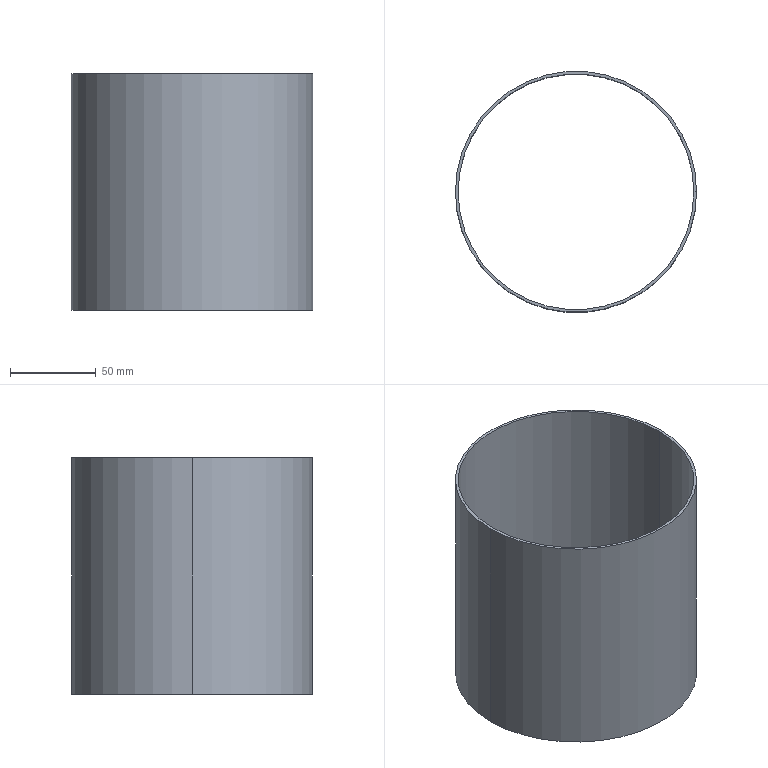Part | SolidWorks | features FlatPattern 1, SMBaseFlange 1, SheetMetal 1 | 1 solid | 8 faces | box 140.5 x 140.5 x 137.6 mm | volume 96049 mm3 | cylinder 4 | plane 4 | commonest cylinder face diameters 137.3 x2 140.5 x2
STEP:
#1=CARTESIAN_POINT('',(68.65,0.04886,137.6));
#2=VERTEX_POINT('',#1);
#3=CARTESIAN_POINT('',(-68.65,0.,137.6));
#4=VERTEX_POINT('',#3);
#5=CARTESIAN_POINT('',(0.,0.,137.6));
#6=DIRECTION('',(0.,0.,1.));
#7=DIRECTION('',(1.,0.,0.));
#8=AXIS2_PLACEMENT_3D('',#5,#6,#7);
#9=CIRCLE('',#8,68.65);
#10=EDGE_CURVE('',#2,#4,#9,.T.);
#11=ORIENTED_EDGE('',*,*,#10,.T.);
#12=CARTESIAN_POINT('',(-68.65,0.,0.));
#13=VERTEX_POINT('',#12);
#14=CARTESIAN_POINT('',(-68.65,0.,137.6));
#15=DIRECTION('',(0.,0.,-1.));
#16=VECTOR('',#15,1000.);
#17=LINE('',#14,#16);
#18=EDGE_CURVE('',#4,#13,#17,.T.);
#19=ORIENTED_EDGE('',*,*,#18,.T.);
#20=CARTESIAN_POINT('',(68.65,0.04886,0.));
#21=VERTEX_POINT('',#20);
#22=CARTESIAN_POINT('',(0.,0.,0.));
#23=DIRECTION('',(0.,0.,1.));
#24=DIRECTION('',(1.,0.,0.));
#25=AXIS2_PLACEMENT_3D('',#22,#23,#24);
#26=CIRCLE('',#25,68.65);
#27=EDGE_CURVE('',#21,#13,#26,.T.);
#28=ORIENTED_EDGE('',*,*,#27,.F.);
#29=CARTESIAN_POINT('',(68.65,0.04886,137.6));
#30=DIRECTION('',(0.,0.,-1.));
#31=VECTOR('',#30,1000.);
#32=LINE('',#29,#31);
#33=EDGE_CURVE('',#2,#21,#32,.T.);
#34=ORIENTED_EDGE('',*,*,#33,.F.);
#35=EDGE_LOOP('',(#11,#19,#28,#34));
#36=FACE_OUTER_BOUND('',#35,.T.);
#37=CARTESIAN_POINT('',(0.,0.,137.6));
#38=DIRECTION('',(0.,0.,-1.));
#39=DIRECTION('',(-1.,0.,0.));
#40=AXIS2_PLACEMENT_3D('',#37,#38,#39);
#41=CYLINDRICAL_SURFACE('',#40,68.65);
#42=ADVANCED_FACE('',(#36),#41,.F.);
#43=CARTESIAN_POINT('',(-70.25,0.,137.6));
#44=VERTEX_POINT('',#43);
#45=CARTESIAN_POINT('',(70.25,-0.05,137.6));
#46=VERTEX_POINT('',#45);
#47=CARTESIAN_POINT('',(0.,0.,137.6));
#48=DIRECTION('',(0.,0.,1.));
#49=DIRECTION('',(1.,0.,0.));
#50=AXIS2_PLACEMENT_3D('',#47,#48,#49);
#51=CIRCLE('',#50,70.25);
#52=EDGE_CURVE('',#44,#46,#51,.T.);
#53=ORIENTED_EDGE('',*,*,#52,.F.);
#54=CARTESIAN_POINT('',(-70.25,0.,0.));
#55=VERTEX_POINT('',#54);
#56=CARTESIAN_POINT('',(-70.25,0.,137.6));
#57=DIRECTION('',(0.,0.,-1.));
#58=VECTOR('',#57,1000.);
#59=LINE('',#56,#58);
#60=EDGE_CURVE('',#44,#55,#59,.T.);
#61=ORIENTED_EDGE('',*,*,#60,.T.);
#62=CARTESIAN_POINT('',(70.25,-0.05,0.));
#63=VERTEX_POINT('',#62);
#64=CARTESIAN_POINT('',(0.,0.,0.));
#65=DIRECTION('',(0.,0.,1.));
#66=DIRECTION('',(1.,0.,0.));
#67=AXIS2_PLACEMENT_3D('',#64,#65,#66);
#68=CIRCLE('',#67,70.25);
#69=EDGE_CURVE('',#55,#63,#68,.T.);
#70=ORIENTED_EDGE('',*,*,#69,.T.);
#71=CARTESIAN_POINT('',(70.25,-0.05,137.6));
#72=DIRECTION('',(0.,0.,-1.));
#73=VECTOR('',#72,1000.);
#74=LINE('',#71,#73);
#75=EDGE_CURVE('',#46,#63,#74,.T.);
#76=ORIENTED_EDGE('',*,*,#75,.F.);
#77=EDGE_LOOP('',(#53,#61,#70,#76));
#78=FACE_OUTER_BOUND('',#77,.T.);
#79=CARTESIAN_POINT('',(0.,0.,137.6));
#80=DIRECTION('',(0.,0.,-1.));
#81=DIRECTION('',(-1.,0.,0.));
#82=AXIS2_PLACEMENT_3D('',#79,#80,#81);
#83=CYLINDRICAL_SURFACE('',#82,70.25);
#84=ADVANCED_FACE('',(#78),#83,.T.);
#85=ORIENTED_EDGE('',*,*,#60,.F.);
#86=CARTESIAN_POINT('',(70.25,0.05,137.6));
#87=VERTEX_POINT('',#86);
#88=CARTESIAN_POINT('',(0.,0.,137.6));
#89=DIRECTION('',(0.,0.,1.));
#90=DIRECTION('',(1.,0.,0.));
#91=AXIS2_PLACEMENT_3D('',#88,#89,#90);
#92=CIRCLE('',#91,70.25);
#93=EDGE_CURVE('',#87,#44,#92,.T.);
#94=ORIENTED_EDGE('',*,*,#93,.F.);
#95=CARTESIAN_POINT('',(70.25,0.05,0.));
#96=VERTEX_POINT('',#95);
#97=CARTESIAN_POINT('',(70.25,0.05,137.6));
#98=DIRECTION('',(0.,0.,-1.));
#99=VECTOR('',#98,1000.);
#100=LINE('',#97,#99);
#101=EDGE_CURVE('',#87,#96,#100,.T.);
#102=ORIENTED_EDGE('',*,*,#101,.T.);
#103=CARTESIAN_POINT('',(0.,0.,0.));
#104=DIRECTION('',(0.,0.,1.));
#105=DIRECTION('',(1.,0.,0.));
#106=AXIS2_PLACEMENT_3D('',#103,#104,#105);
#107=CIRCLE('',#106,70.25);
#108=EDGE_CURVE('',#96,#55,#107,.T.);
#109=ORIENTED_EDGE('',*,*,#108,.T.);
#110=EDGE_LOOP('',(#85,#94,#102,#109));
#111=FACE_OUTER_BOUND('',#110,.T.);
#112=CARTESIAN_POINT('',(0.,0.,137.6));
#113=DIRECTION('',(0.,0.,-1.));
#114=DIRECTION('',(-1.,0.,0.));
#115=AXIS2_PLACEMENT_3D('',#112,#113,#114);
#116=CYLINDRICAL_SURFACE('',#115,70.25);
#117=ADVANCED_FACE('',(#111),#116,.T.);
#118=CARTESIAN_POINT('',(68.65,-0.04886,0.));
#119=VERTEX_POINT('',#118);
#120=CARTESIAN_POINT('',(68.65,-0.04886,0.));
#121=DIRECTION('',(1.,-0.0007117,0.));
#122=VECTOR('',#121,1000.);
#123=LINE('',#120,#122);
#124=EDGE_CURVE('',#119,#63,#123,.T.);
#125=ORIENTED_EDGE('',*,*,#124,.F.);
#126=CARTESIAN_POINT('',(68.65,-0.04886,137.6));
#127=VERTEX_POINT('',#126);
#128=CARTESIAN_POINT('',(68.65,-0.04886,137.6));
#129=DIRECTION('',(0.,0.,-1.));
#130=VECTOR('',#129,1000.);
#131=LINE('',#128,#130);
#132=EDGE_CURVE('',#127,#119,#131,.T.);
#133=ORIENTED_EDGE('',*,*,#132,.F.);
#134=CARTESIAN_POINT('',(68.65,-0.04886,137.6));
#135=DIRECTION('',(1.,-0.0007117,0.));
#136=VECTOR('',#135,1000.);
#137=LINE('',#134,#136);
#138=EDGE_CURVE('',#127,#46,#137,.T.);
#139=ORIENTED_EDGE('',*,*,#138,.T.);
#140=ORIENTED_EDGE('',*,*,#75,.T.);
#141=EDGE_LOOP('',(#125,#133,#139,#140));
#142=FACE_OUTER_BOUND('',#141,.T.);
#143=CARTESIAN_POINT('',(68.65,-0.04886,137.6));
#144=DIRECTION('',(0.0007117,1.,0.));
#145=DIRECTION('',(-1.,0.0007117,0.));
#146=AXIS2_PLACEMENT_3D('',#143,#144,#145);
#147=PLANE('',#146);
#148=ADVANCED_FACE('',(#142),#147,.T.);
#149=ORIENTED_EDGE('',*,*,#18,.F.);
#150=CARTESIAN_POINT('',(0.,0.,137.6));
#151=DIRECTION('',(0.,0.,1.));
#152=DIRECTION('',(1.,0.,0.));
#153=AXIS2_PLACEMENT_3D('',#150,#151,#152);
#154=CIRCLE('',#153,68.65);
#155=EDGE_CURVE('',#4,#127,#154,.T.);
#156=ORIENTED_EDGE('',*,*,#155,.T.);
#157=ORIENTED_EDGE('',*,*,#132,.T.);
#158=CARTESIAN_POINT('',(0.,0.,0.));
#159=DIRECTION('',(0.,0.,1.));
#160=DIRECTION('',(1.,0.,0.));
#161=AXIS2_PLACEMENT_3D('',#158,#159,#160);
#162=CIRCLE('',#161,68.65);
#163=EDGE_CURVE('',#13,#119,#162,.T.);
#164=ORIENTED_EDGE('',*,*,#163,.F.);
#165=EDGE_LOOP('',(#149,#156,#157,#164));
#166=FACE_OUTER_BOUND('',#165,.T.);
#167=CARTESIAN_POINT('',(0.,0.,137.6));
#168=DIRECTION('',(0.,0.,-1.));
#169=DIRECTION('',(-1.,0.,0.));
#170=AXIS2_PLACEMENT_3D('',#167,#168,#169);
#171=CYLINDRICAL_SURFACE('',#170,68.65);
#172=ADVANCED_FACE('',(#166),#171,.F.);
#173=CARTESIAN_POINT('',(70.25,0.05,0.));
#174=DIRECTION('',(-1.,-0.0007117,0.));
#175=VECTOR('',#174,1000.);
#176=LINE('',#173,#175);
#177=EDGE_CURVE('',#96,#21,#176,.T.);
#178=ORIENTED_EDGE('',*,*,#177,.F.);
#179=ORIENTED_EDGE('',*,*,#101,.F.);
#180=CARTESIAN_POINT('',(70.25,0.05,137.6));
#181=DIRECTION('',(-1.,-0.0007117,0.));
#182=VECTOR('',#181,1000.);
#183=LINE('',#180,#182);
#184=EDGE_CURVE('',#87,#2,#183,.T.);
#185=ORIENTED_EDGE('',*,*,#184,.T.);
#186=ORIENTED_EDGE('',*,*,#33,.T.);
#187=EDGE_LOOP('',(#178,#179,#185,#186));
#188=FACE_OUTER_BOUND('',#187,.T.);
#189=CARTESIAN_POINT('',(70.25,0.05,137.6));
#190=DIRECTION('',(0.0007117,-1.,0.));
#191=DIRECTION('',(1.,0.0007117,0.));
#192=AXIS2_PLACEMENT_3D('',#189,#190,#191);
#193=PLANE('',#192);
#194=ADVANCED_FACE('',(#188),#193,.T.);
#195=ORIENTED_EDGE('',*,*,#93,.T.);
#196=ORIENTED_EDGE('',*,*,#52,.T.);
#197=ORIENTED_EDGE('',*,*,#138,.F.);
#198=ORIENTED_EDGE('',*,*,#155,.F.);
#199=ORIENTED_EDGE('',*,*,#10,.F.);
#200=ORIENTED_EDGE('',*,*,#184,.F.);
#201=EDGE_LOOP('',(#195,#196,#197,#198,#199,#200));
#202=FACE_OUTER_BOUND('',#201,.T.);
#203=CARTESIAN_POINT('',(0.,0.,137.6));
#204=DIRECTION('',(0.,0.,1.));
#205=DIRECTION('',(1.,0.,0.));
#206=AXIS2_PLACEMENT_3D('',#203,#204,#205);
#207=PLANE('',#206);
#208=ADVANCED_FACE('',(#202),#207,.T.);
#209=ORIENTED_EDGE('',*,*,#108,.F.);
#210=ORIENTED_EDGE('',*,*,#177,.T.);
#211=ORIENTED_EDGE('',*,*,#27,.T.);
#212=ORIENTED_EDGE('',*,*,#163,.T.);
#213=ORIENTED_EDGE('',*,*,#124,.T.);
#214=ORIENTED_EDGE('',*,*,#69,.F.);
#215=EDGE_LOOP('',(#209,#210,#211,#212,#213,#214));
#216=FACE_OUTER_BOUND('',#215,.T.);
#217=CARTESIAN_POINT('',(0.,0.,0.));
#218=DIRECTION('',(0.,0.,1.));
#219=DIRECTION('',(1.,0.,0.));
#220=AXIS2_PLACEMENT_3D('',#217,#218,#219);
#221=PLANE('',#220);
#222=ADVANCED_FACE('',(#216),#221,.F.);
#223=CLOSED_SHELL('',(#42,#84,#117,#148,#172,#194,#208,#222));
#224=MANIFOLD_SOLID_BREP('',#223);
#225=CARTESIAN_POINT('',(0.,0.,0.));
#226=DIRECTION('',(0.,0.,1.));
#227=DIRECTION('',(1.,0.,0.));
#228=AXIS2_PLACEMENT_3D('',#225,#226,#227);
#229=(LENGTH_UNIT()NAMED_UNIT(*)SI_UNIT(.MILLI.,.METRE.));
#230=UNCERTAINTY_MEASURE_WITH_UNIT(LENGTH_MEASURE(0.00001),#229,'','');
#231=(NAMED_UNIT(*)PLANE_ANGLE_UNIT()SI_UNIT($,.RADIAN.));
#232=(NAMED_UNIT(*)SI_UNIT($,.STERADIAN.)SOLID_ANGLE_UNIT());
#233=(GEOMETRIC_REPRESENTATION_CONTEXT(3)GLOBAL_UNCERTAINTY_ASSIGNED_CONTEXT((#230))GLOBAL_UNIT_ASSIGNED_CONTEXT((#229,#231,#232))REPRESENTATION_CONTEXT('',''));
#234=ADVANCED_BREP_SHAPE_REPRESENTATION('',(#224,#228),#233);